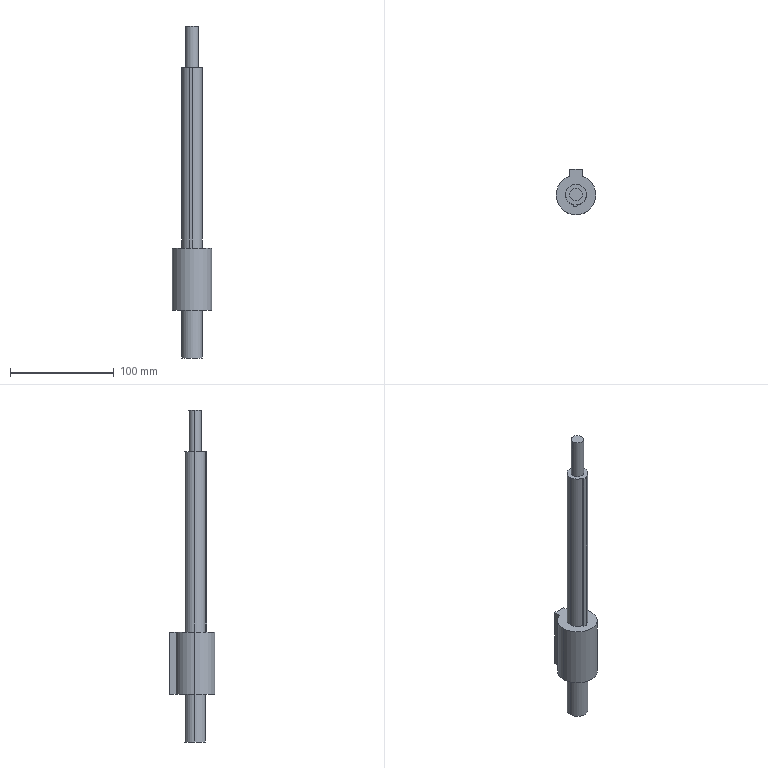Part | STEP file | Camshaft | 1 solid | 21 faces | box 38.228 x 43.828 x 320 mm | volume 147567 mm3 | plane 11 | cylinder 10 | commonest cylinder face diameters 20 x5 38.228 x3 12 x2
STEP:
#1=CARTESIAN_POINT('',(0.,0.,0.));
#2=DIRECTION('',(0.,0.,1.));
#3=DIRECTION('',(1.,0.,0.));
#4=AXIS2_PLACEMENT_3D('',#1,#2,#3);
#5=CARTESIAN_POINT('',(-50.965,1.642,236.173));
#6=VERTEX_POINT('',#5);
#7=CARTESIAN_POINT('',(-62.965,1.642,236.173));
#8=VERTEX_POINT('',#7);
#9=CARTESIAN_POINT('',(-56.965,1.642,236.173));
#10=DIRECTION('',(0.,0.,1.));
#11=DIRECTION('',(1.,0.,0.));
#12=AXIS2_PLACEMENT_3D('',#9,#10,#11);
#13=CIRCLE('',#12,6.);
#14=CARTESIAN_POINT('',(-56.965,1.642,236.173));
#15=DIRECTION('',(0.,0.,-1.));
#16=DIRECTION('',(-1.,0.,0.));
#17=AXIS2_PLACEMENT_3D('',#14,#15,#16);
#18=CYLINDRICAL_SURFACE('',#17,6.);
#19=CARTESIAN_POINT('',(3.142,0.));
#20=DIRECTION('',(-1.,0.));
#21=VECTOR('',#20,1.);
#22=LINE('',#19,#21);
#23=(GEOMETRIC_REPRESENTATION_CONTEXT(2)PARAMETRIC_REPRESENTATION_CONTEXT()REPRESENTATION_CONTEXT('',''));
#24=DEFINITIONAL_REPRESENTATION('',(#22),#23);
#25=PCURVE('',#18,#24);
#26=CARTESIAN_POINT('',(-56.965,1.642,236.173));
#27=DIRECTION('',(0.,0.,1.));
#28=DIRECTION('',(1.,0.,0.));
#29=AXIS2_PLACEMENT_3D('',#26,#27,#28);
#30=PLANE('',#29);
#31=CARTESIAN_POINT('',(0.,0.));
#32=DIRECTION('',(1.,0.));
#33=AXIS2_PLACEMENT_2D('',#31,#32);
#34=CIRCLE('',#33,6.);
#35=(GEOMETRIC_REPRESENTATION_CONTEXT(2)PARAMETRIC_REPRESENTATION_CONTEXT()REPRESENTATION_CONTEXT('',''));
#36=DEFINITIONAL_REPRESENTATION('',(#34),#35);
#37=PCURVE('',#30,#36);
#38=SURFACE_CURVE('',#13,(#25,#37),.PCURVE_S1.);
#39=EDGE_CURVE('',#6,#8,#38,.T.);
#40=ORIENTED_EDGE('',*,*,#39,.F.);
#41=CARTESIAN_POINT('',(-50.965,1.642,196.173));
#42=VERTEX_POINT('',#41);
#43=CARTESIAN_POINT('',(-50.965,1.642,236.173));
#44=DIRECTION('',(0.,0.,-1.));
#45=VECTOR('',#44,1.);
#46=LINE('',#43,#45);
#47=CARTESIAN_POINT('',(3.142,0.));
#48=DIRECTION('',(0.,1.));
#49=VECTOR('',#48,1.);
#50=LINE('',#47,#49);
#51=(GEOMETRIC_REPRESENTATION_CONTEXT(2)PARAMETRIC_REPRESENTATION_CONTEXT()REPRESENTATION_CONTEXT('',''));
#52=DEFINITIONAL_REPRESENTATION('',(#50),#51);
#53=PCURVE('',#18,#52);
#54=CARTESIAN_POINT('',(-56.965,1.642,236.173));
#55=DIRECTION('',(0.,0.,-1.));
#56=DIRECTION('',(-1.,0.,0.));
#57=AXIS2_PLACEMENT_3D('',#54,#55,#56);
#58=CYLINDRICAL_SURFACE('',#57,6.);
#59=CARTESIAN_POINT('',(3.142,0.));
#60=DIRECTION('',(0.,1.));
#61=VECTOR('',#60,1.);
#62=LINE('',#59,#61);
#63=(GEOMETRIC_REPRESENTATION_CONTEXT(2)PARAMETRIC_REPRESENTATION_CONTEXT()REPRESENTATION_CONTEXT('',''));
#64=DEFINITIONAL_REPRESENTATION('',(#62),#63);
#65=PCURVE('',#58,#64);
#66=SURFACE_CURVE('',#46,(#53,#65),.PCURVE_S1.);
#67=EDGE_CURVE('',#6,#42,#66,.T.);
#68=ORIENTED_EDGE('',*,*,#67,.T.);
#69=CARTESIAN_POINT('',(-62.965,1.642,196.173));
#70=VERTEX_POINT('',#69);
#71=CARTESIAN_POINT('',(-56.965,1.642,196.173));
#72=DIRECTION('',(0.,0.,1.));
#73=DIRECTION('',(1.,0.,0.));
#74=AXIS2_PLACEMENT_3D('',#71,#72,#73);
#75=CIRCLE('',#74,6.);
#76=CARTESIAN_POINT('',(3.142,40.));
#77=DIRECTION('',(-1.,0.));
#78=VECTOR('',#77,1.);
#79=LINE('',#76,#78);
#80=(GEOMETRIC_REPRESENTATION_CONTEXT(2)PARAMETRIC_REPRESENTATION_CONTEXT()REPRESENTATION_CONTEXT('',''));
#81=DEFINITIONAL_REPRESENTATION('',(#79),#80);
#82=PCURVE('',#18,#81);
#83=CARTESIAN_POINT('',(-56.965,1.642,196.173));
#84=DIRECTION('',(0.,0.,1.));
#85=DIRECTION('',(1.,0.,0.));
#86=AXIS2_PLACEMENT_3D('',#83,#84,#85);
#87=PLANE('',#86);
#88=CARTESIAN_POINT('',(0.,0.));
#89=DIRECTION('',(1.,0.));
#90=AXIS2_PLACEMENT_2D('',#88,#89);
#91=CIRCLE('',#90,6.);
#92=(GEOMETRIC_REPRESENTATION_CONTEXT(2)PARAMETRIC_REPRESENTATION_CONTEXT()REPRESENTATION_CONTEXT('',''));
#93=DEFINITIONAL_REPRESENTATION('',(#91),#92);
#94=PCURVE('',#87,#93);
#95=SURFACE_CURVE('',#75,(#82,#94),.PCURVE_S1.);
#96=EDGE_CURVE('',#42,#70,#95,.T.);
#97=ORIENTED_EDGE('',*,*,#96,.T.);
#98=CARTESIAN_POINT('',(-62.965,1.642,236.173));
#99=DIRECTION('',(0.,0.,-1.));
#100=VECTOR('',#99,1.);
#101=LINE('',#98,#100);
#102=CARTESIAN_POINT('',(0.,0.));
#103=DIRECTION('',(0.,1.));
#104=VECTOR('',#103,1.);
#105=LINE('',#102,#104);
#106=(GEOMETRIC_REPRESENTATION_CONTEXT(2)PARAMETRIC_REPRESENTATION_CONTEXT()REPRESENTATION_CONTEXT('',''));
#107=DEFINITIONAL_REPRESENTATION('',(#105),#106);
#108=PCURVE('',#18,#107);
#109=CARTESIAN_POINT('',(6.283,0.));
#110=DIRECTION('',(0.,1.));
#111=VECTOR('',#110,1.);
#112=LINE('',#109,#111);
#113=(GEOMETRIC_REPRESENTATION_CONTEXT(2)PARAMETRIC_REPRESENTATION_CONTEXT()REPRESENTATION_CONTEXT('',''));
#114=DEFINITIONAL_REPRESENTATION('',(#112),#113);
#115=PCURVE('',#58,#114);
#116=SURFACE_CURVE('',#101,(#108,#115),.PCURVE_S1.);
#117=EDGE_CURVE('',#8,#70,#116,.T.);
#118=ORIENTED_EDGE('',*,*,#117,.F.);
#119=EDGE_LOOP('',(#40,#68,#97,#118));
#120=FACE_BOUND('',#119,.T.);
#121=ADVANCED_FACE('',(#120),#18,.T.);
#122=CARTESIAN_POINT('',(-46.965,1.642,22.173));
#123=VERTEX_POINT('',#122);
#124=CARTESIAN_POINT('',(-66.965,1.642,22.173));
#125=VERTEX_POINT('',#124);
#126=CARTESIAN_POINT('',(-56.965,1.642,22.173));
#127=DIRECTION('',(0.,0.,1.));
#128=DIRECTION('',(1.,0.,0.));
#129=AXIS2_PLACEMENT_3D('',#126,#127,#128);
#130=CIRCLE('',#129,10.);
#131=CARTESIAN_POINT('',(-56.965,1.642,-83.827));
#132=DIRECTION('',(0.,0.,1.));
#133=DIRECTION('',(1.,0.,0.));
#134=AXIS2_PLACEMENT_3D('',#131,#132,#133);
#135=CYLINDRICAL_SURFACE('',#134,10.);
#136=CARTESIAN_POINT('',(0.,106.));
#137=DIRECTION('',(1.,0.));
#138=VECTOR('',#137,1.);
#139=LINE('',#136,#138);
#140=(GEOMETRIC_REPRESENTATION_CONTEXT(2)PARAMETRIC_REPRESENTATION_CONTEXT()REPRESENTATION_CONTEXT('',''));
#141=DEFINITIONAL_REPRESENTATION('',(#139),#140);
#142=PCURVE('',#135,#141);
#143=CARTESIAN_POINT('',(-56.965,1.642,22.173));
#144=DIRECTION('',(0.,0.,1.));
#145=DIRECTION('',(1.,0.,0.));
#146=AXIS2_PLACEMENT_3D('',#143,#144,#145);
#147=PLANE('',#146);
#148=CARTESIAN_POINT('',(0.,0.));
#149=DIRECTION('',(1.,0.));
#150=AXIS2_PLACEMENT_2D('',#148,#149);
#151=CIRCLE('',#150,10.);
#152=(GEOMETRIC_REPRESENTATION_CONTEXT(2)PARAMETRIC_REPRESENTATION_CONTEXT()REPRESENTATION_CONTEXT('',''));
#153=DEFINITIONAL_REPRESENTATION('',(#151),#152);
#154=PCURVE('',#147,#153);
#155=SURFACE_CURVE('',#130,(#142,#154),.PCURVE_S1.);
#156=EDGE_CURVE('',#123,#125,#155,.T.);
#157=ORIENTED_EDGE('',*,*,#156,.T.);
#158=CARTESIAN_POINT('',(-66.965,1.642,196.173));
#159=VERTEX_POINT('',#158);
#160=CARTESIAN_POINT('',(-66.965,1.642,-83.827));
#161=DIRECTION('',(0.,0.,1.));
#162=VECTOR('',#161,1.);
#163=LINE('',#160,#162);
#164=CARTESIAN_POINT('',(3.142,0.));
#165=DIRECTION('',(0.,1.));
#166=VECTOR('',#165,1.);
#167=LINE('',#164,#166);
#168=(GEOMETRIC_REPRESENTATION_CONTEXT(2)PARAMETRIC_REPRESENTATION_CONTEXT()REPRESENTATION_CONTEXT('',''));
#169=DEFINITIONAL_REPRESENTATION('',(#167),#168);
#170=PCURVE('',#135,#169);
#171=CARTESIAN_POINT('',(-56.965,1.642,-83.827));
#172=DIRECTION('',(0.,0.,1.));
#173=DIRECTION('',(1.,0.,0.));
#174=AXIS2_PLACEMENT_3D('',#171,#172,#173);
#175=CYLINDRICAL_SURFACE('',#174,10.);
#176=CARTESIAN_POINT('',(3.142,0.));
#177=DIRECTION('',(0.,1.));
#178=VECTOR('',#177,1.);
#179=LINE('',#176,#178);
#180=(GEOMETRIC_REPRESENTATION_CONTEXT(2)PARAMETRIC_REPRESENTATION_CONTEXT()REPRESENTATION_CONTEXT('',''));
#181=DEFINITIONAL_REPRESENTATION('',(#179),#180);
#182=PCURVE('',#175,#181);
#183=SURFACE_CURVE('',#163,(#170,#182),.PCURVE_S1.);
#184=EDGE_CURVE('',#125,#159,#183,.T.);
#185=ORIENTED_EDGE('',*,*,#184,.T.);
#186=CARTESIAN_POINT('',(-46.965,1.642,196.173));
#187=VERTEX_POINT('',#186);
#188=CARTESIAN_POINT('',(-56.965,1.642,196.173));
#189=DIRECTION('',(0.,0.,1.));
#190=DIRECTION('',(1.,0.,0.));
#191=AXIS2_PLACEMENT_3D('',#188,#189,#190);
#192=CIRCLE('',#191,10.);
#193=CARTESIAN_POINT('',(0.,280.));
#194=DIRECTION('',(1.,0.));
#195=VECTOR('',#194,1.);
#196=LINE('',#193,#195);
#197=(GEOMETRIC_REPRESENTATION_CONTEXT(2)PARAMETRIC_REPRESENTATION_CONTEXT()REPRESENTATION_CONTEXT('',''));
#198=DEFINITIONAL_REPRESENTATION('',(#196),#197);
#199=PCURVE('',#135,#198);
#200=CARTESIAN_POINT('',(0.,0.));
#201=DIRECTION('',(1.,0.));
#202=AXIS2_PLACEMENT_2D('',#200,#201);
#203=CIRCLE('',#202,10.);
#204=(GEOMETRIC_REPRESENTATION_CONTEXT(2)PARAMETRIC_REPRESENTATION_CONTEXT()REPRESENTATION_CONTEXT('',''));
#205=DEFINITIONAL_REPRESENTATION('',(#203),#204);
#206=PCURVE('',#87,#205);
#207=SURFACE_CURVE('',#192,(#199,#206),.PCURVE_S1.);
#208=EDGE_CURVE('',#187,#159,#207,.T.);
#209=ORIENTED_EDGE('',*,*,#208,.F.);
#210=CARTESIAN_POINT('',(-46.965,1.642,-83.827));
#211=DIRECTION('',(0.,0.,1.));
#212=VECTOR('',#211,1.);
#213=LINE('',#210,#212);
#214=CARTESIAN_POINT('',(0.,0.));
#215=DIRECTION('',(0.,1.));
#216=VECTOR('',#215,1.);
#217=LINE('',#214,#216);
#218=(GEOMETRIC_REPRESENTATION_CONTEXT(2)PARAMETRIC_REPRESENTATION_CONTEXT()REPRESENTATION_CONTEXT('',''));
#219=DEFINITIONAL_REPRESENTATION('',(#217),#218);
#220=PCURVE('',#135,#219);
#221=CARTESIAN_POINT('',(-56.965,1.642,-83.827));
#222=DIRECTION('',(0.,0.,1.));
#223=DIRECTION('',(1.,0.,0.));
#224=AXIS2_PLACEMENT_3D('',#221,#222,#223);
#225=CYLINDRICAL_SURFACE('',#224,10.);
#226=CARTESIAN_POINT('',(6.283,0.));
#227=DIRECTION('',(0.,1.));
#228=VECTOR('',#227,1.);
#229=LINE('',#226,#228);
#230=(GEOMETRIC_REPRESENTATION_CONTEXT(2)PARAMETRIC_REPRESENTATION_CONTEXT()REPRESENTATION_CONTEXT('',''));
#231=DEFINITIONAL_REPRESENTATION('',(#229),#230);
#232=PCURVE('',#225,#231);
#233=SURFACE_CURVE('',#213,(#220,#232),.PCURVE_S1.);
#234=EDGE_CURVE('',#123,#187,#233,.T.);
#235=ORIENTED_EDGE('',*,*,#234,.F.);
#236=EDGE_LOOP('',(#157,#185,#209,#235));
#237=FACE_BOUND('',#236,.T.);
#238=ADVANCED_FACE('',(#237),#135,.T.);
#239=CARTESIAN_POINT('',(-56.27,-8.334,22.173));
#240=VERTEX_POINT('',#239);
#241=CARTESIAN_POINT('',(-56.965,1.642,22.173));
#242=DIRECTION('',(0.,0.,1.));
#243=DIRECTION('',(1.,0.,0.));
#244=AXIS2_PLACEMENT_3D('',#241,#242,#243);
#245=CIRCLE('',#244,10.);
#246=CARTESIAN_POINT('',(0.,106.));
#247=DIRECTION('',(1.,0.));
#248=VECTOR('',#247,1.);
#249=LINE('',#246,#248);
#250=(GEOMETRIC_REPRESENTATION_CONTEXT(2)PARAMETRIC_REPRESENTATION_CONTEXT()REPRESENTATION_CONTEXT('',''));
#251=DEFINITIONAL_REPRESENTATION('',(#249),#250);
#252=PCURVE('',#225,#251);
#253=CARTESIAN_POINT('',(0.,0.));
#254=DIRECTION('',(1.,0.));
#255=AXIS2_PLACEMENT_2D('',#253,#254);
#256=CIRCLE('',#255,10.);
#257=(GEOMETRIC_REPRESENTATION_CONTEXT(2)PARAMETRIC_REPRESENTATION_CONTEXT()REPRESENTATION_CONTEXT('',''));
#258=DEFINITIONAL_REPRESENTATION('',(#256),#257);
#259=PCURVE('',#147,#258);
#260=SURFACE_CURVE('',#245,(#252,#259),.PCURVE_S1.);
#261=EDGE_CURVE('',#240,#123,#260,.T.);
#262=ORIENTED_EDGE('',*,*,#261,.T.);
#263=ORIENTED_EDGE('',*,*,#234,.T.);
#264=CARTESIAN_POINT('',(-56.27,-8.334,196.173));
#265=VERTEX_POINT('',#264);
#266=CARTESIAN_POINT('',(-56.965,1.642,196.173));
#267=DIRECTION('',(0.,0.,1.));
#268=DIRECTION('',(1.,0.,0.));
#269=AXIS2_PLACEMENT_3D('',#266,#267,#268);
#270=CIRCLE('',#269,10.);
#271=CARTESIAN_POINT('',(0.,280.));
#272=DIRECTION('',(1.,0.));
#273=VECTOR('',#272,1.);
#274=LINE('',#271,#273);
#275=(GEOMETRIC_REPRESENTATION_CONTEXT(2)PARAMETRIC_REPRESENTATION_CONTEXT()REPRESENTATION_CONTEXT('',''));
#276=DEFINITIONAL_REPRESENTATION('',(#274),#275);
#277=PCURVE('',#225,#276);
#278=CARTESIAN_POINT('',(0.,0.));
#279=DIRECTION('',(1.,0.));
#280=AXIS2_PLACEMENT_2D('',#278,#279);
#281=CIRCLE('',#280,10.);
#282=(GEOMETRIC_REPRESENTATION_CONTEXT(2)PARAMETRIC_REPRESENTATION_CONTEXT()REPRESENTATION_CONTEXT('',''));
#283=DEFINITIONAL_REPRESENTATION('',(#281),#282);
#284=PCURVE('',#87,#283);
#285=SURFACE_CURVE('',#270,(#277,#284),.PCURVE_S1.);
#286=EDGE_CURVE('',#265,#187,#285,.T.);
#287=ORIENTED_EDGE('',*,*,#286,.F.);
#288=CARTESIAN_POINT('',(-56.27,-8.334,-83.827));
#289=DIRECTION('',(0.,0.,1.));
#290=VECTOR('',#289,1.);
#291=LINE('',#288,#290);
#292=CARTESIAN_POINT('',(4.782,0.));
#293=DIRECTION('',(0.,1.));
#294=VECTOR('',#293,1.);
#295=LINE('',#292,#294);
#296=(GEOMETRIC_REPRESENTATION_CONTEXT(2)PARAMETRIC_REPRESENTATION_CONTEXT()REPRESENTATION_CONTEXT('',''));
#297=DEFINITIONAL_REPRESENTATION('',(#295),#296);
#298=PCURVE('',#225,#297);
#299=CARTESIAN_POINT('',(-56.401,-9.942,9.172));
#300=DIRECTION('',(0.9967,-0.08093,0.));
#301=DIRECTION('',(0.08093,0.9967,0.));
#302=AXIS2_PLACEMENT_3D('',#299,#300,#301);
#303=PLANE('',#302);
#304=CARTESIAN_POINT('',(1.613,-92.999));
#305=DIRECTION('',(0.,1.));
#306=VECTOR('',#305,1.);
#307=LINE('',#304,#306);
#308=(GEOMETRIC_REPRESENTATION_CONTEXT(2)PARAMETRIC_REPRESENTATION_CONTEXT()REPRESENTATION_CONTEXT('',''));
#309=DEFINITIONAL_REPRESENTATION('',(#307),#308);
#310=PCURVE('',#303,#309);
#311=SURFACE_CURVE('',#291,(#298,#310),.PCURVE_S1.);
#312=EDGE_CURVE('',#240,#265,#311,.T.);
#313=ORIENTED_EDGE('',*,*,#312,.F.);
#314=EDGE_LOOP('',(#262,#263,#287,#313));
#315=FACE_BOUND('',#314,.T.);
#316=ADVANCED_FACE('',(#315),#225,.T.);
#317=CARTESIAN_POINT('',(-46.965,1.642,-83.827));
#318=VERTEX_POINT('',#317);
#319=CARTESIAN_POINT('',(-66.965,1.642,-83.827));
#320=VERTEX_POINT('',#319);
#321=CARTESIAN_POINT('',(-56.965,1.642,-83.827));
#322=DIRECTION('',(0.,0.,1.));
#323=DIRECTION('',(1.,0.,0.));
#324=AXIS2_PLACEMENT_3D('',#321,#322,#323);
#325=CIRCLE('',#324,10.);
#326=CARTESIAN_POINT('',(-56.965,1.642,-83.827));
#327=DIRECTION('',(0.,0.,1.));
#328=DIRECTION('',(1.,0.,0.));
#329=AXIS2_PLACEMENT_3D('',#326,#327,#328);
#330=CYLINDRICAL_SURFACE('',#329,10.);
#331=CARTESIAN_POINT('',(0.,0.));
#332=DIRECTION('',(1.,0.));
#333=VECTOR('',#332,1.);
#334=LINE('',#331,#333);
#335=(GEOMETRIC_REPRESENTATION_CONTEXT(2)PARAMETRIC_REPRESENTATION_CONTEXT()REPRESENTATION_CONTEXT('',''));
#336=DEFINITIONAL_REPRESENTATION('',(#334),#335);
#337=PCURVE('',#330,#336);
#338=CARTESIAN_POINT('',(-56.965,1.642,-83.827));
#339=DIRECTION('',(0.,0.,1.));
#340=DIRECTION('',(1.,0.,0.));
#341=AXIS2_PLACEMENT_3D('',#338,#339,#340);
#342=PLANE('',#341);
#343=CARTESIAN_POINT('',(0.,0.));
#344=DIRECTION('',(1.,0.));
#345=AXIS2_PLACEMENT_2D('',#343,#344);
#346=CIRCLE('',#345,10.);
#347=(GEOMETRIC_REPRESENTATION_CONTEXT(2)PARAMETRIC_REPRESENTATION_CONTEXT()REPRESENTATION_CONTEXT('',''));
#348=DEFINITIONAL_REPRESENTATION('',(#346),#347);
#349=PCURVE('',#342,#348);
#350=SURFACE_CURVE('',#325,(#337,#349),.PCURVE_S1.);
#351=EDGE_CURVE('',#318,#320,#350,.T.);
#352=ORIENTED_EDGE('',*,*,#351,.T.);
#353=CARTESIAN_POINT('',(-66.965,1.642,-37.827));
#354=VERTEX_POINT('',#353);
#355=CARTESIAN_POINT('',(-66.965,1.642,-83.827));
#356=DIRECTION('',(0.,0.,1.));
#357=VECTOR('',#356,1.);
#358=LINE('',#355,#357);
#359=CARTESIAN_POINT('',(3.142,0.));
#360=DIRECTION('',(0.,1.));
#361=VECTOR('',#360,1.);
#362=LINE('',#359,#361);
#363=(GEOMETRIC_REPRESENTATION_CONTEXT(2)PARAMETRIC_REPRESENTATION_CONTEXT()REPRESENTATION_CONTEXT('',''));
#364=DEFINITIONAL_REPRESENTATION('',(#362),#363);
#365=PCURVE('',#330,#364);
#366=CARTESIAN_POINT('',(-56.965,1.642,-83.827));
#367=DIRECTION('',(0.,0.,1.));
#368=DIRECTION('',(1.,0.,0.));
#369=AXIS2_PLACEMENT_3D('',#366,#367,#368);
#370=CYLINDRICAL_SURFACE('',#369,10.);
#371=CARTESIAN_POINT('',(3.142,0.));
#372=DIRECTION('',(0.,1.));
#373=VECTOR('',#372,1.);
#374=LINE('',#371,#373);
#375=(GEOMETRIC_REPRESENTATION_CONTEXT(2)PARAMETRIC_REPRESENTATION_CONTEXT()REPRESENTATION_CONTEXT('',''));
#376=DEFINITIONAL_REPRESENTATION('',(#374),#375);
#377=PCURVE('',#370,#376);
#378=SURFACE_CURVE('',#358,(#365,#377),.PCURVE_S1.);
#379=EDGE_CURVE('',#320,#354,#378,.T.);
#380=ORIENTED_EDGE('',*,*,#379,.T.);
#381=CARTESIAN_POINT('',(-46.965,1.642,-37.827));
#382=VERTEX_POINT('',#381);
#383=CARTESIAN_POINT('',(-56.965,1.642,-37.827));
#384=DIRECTION('',(0.,0.,1.));
#385=DIRECTION('',(1.,0.,0.));
#386=AXIS2_PLACEMENT_3D('',#383,#384,#385);
#387=CIRCLE('',#386,10.);
#388=CARTESIAN_POINT('',(0.,46.));
#389=DIRECTION('',(1.,0.));
#390=VECTOR('',#389,1.);
#391=LINE('',#388,#390);
#392=(GEOMETRIC_REPRESENTATION_CONTEXT(2)PARAMETRIC_REPRESENTATION_CONTEXT()REPRESENTATION_CONTEXT('',''));
#393=DEFINITIONAL_REPRESENTATION('',(#391),#392);
#394=PCURVE('',#330,#393);
#395=CARTESIAN_POINT('',(-56.965,1.642,-37.827));
#396=DIRECTION('',(0.,0.,1.));
#397=DIRECTION('',(1.,0.,0.));
#398=AXIS2_PLACEMENT_3D('',#395,#396,#397);
#399=PLANE('',#398);
#400=CARTESIAN_POINT('',(0.,0.));
#401=DIRECTION('',(1.,0.));
#402=AXIS2_PLACEMENT_2D('',#400,#401);
#403=CIRCLE('',#402,10.);
#404=(GEOMETRIC_REPRESENTATION_CONTEXT(2)PARAMETRIC_REPRESENTATION_CONTEXT()REPRESENTATION_CONTEXT('',''));
#405=DEFINITIONAL_REPRESENTATION('',(#403),#404);
#406=PCURVE('',#399,#405);
#407=SURFACE_CURVE('',#387,(#394,#406),.PCURVE_S1.);
#408=EDGE_CURVE('',#382,#354,#407,.T.);
#409=ORIENTED_EDGE('',*,*,#408,.F.);
#410=CARTESIAN_POINT('',(-46.965,1.642,-83.827));
#411=DIRECTION('',(0.,0.,1.));
#412=VECTOR('',#411,1.);
#413=LINE('',#410,#412);
#414=CARTESIAN_POINT('',(0.,0.));
#415=DIRECTION('',(0.,1.));
#416=VECTOR('',#415,1.);
#417=LINE('',#414,#416);
#418=(GEOMETRIC_REPRESENTATION_CONTEXT(2)PARAMETRIC_REPRESENTATION_CONTEXT()REPRESENTATION_CONTEXT('',''));
#419=DEFINITIONAL_REPRESENTATION('',(#417),#418);
#420=PCURVE('',#330,#419);
#421=CARTESIAN_POINT('',(6.283,0.));
#422=DIRECTION('',(0.,1.));
#423=VECTOR('',#422,1.);
#424=LINE('',#421,#423);
#425=(GEOMETRIC_REPRESENTATION_CONTEXT(2)PARAMETRIC_REPRESENTATION_CONTEXT()REPRESENTATION_CONTEXT('',''));
#426=DEFINITIONAL_REPRESENTATION('',(#424),#425);
#427=PCURVE('',#370,#426);
#428=SURFACE_CURVE('',#413,(#420,#427),.PCURVE_S1.);
#429=EDGE_CURVE('',#318,#382,#428,.T.);
#430=ORIENTED_EDGE('',*,*,#429,.F.);
#431=EDGE_LOOP('',(#352,#380,#409,#430));
#432=FACE_BOUND('',#431,.T.);
#433=ADVANCED_FACE('',(#432),#330,.T.);
#434=CARTESIAN_POINT('',(-37.851,1.642,22.173));
#435=VERTEX_POINT('',#434);
#436=CARTESIAN_POINT('',(-50.965,19.79,22.173));
#437=VERTEX_POINT('',#436);
#438=CARTESIAN_POINT('',(-56.965,1.642,22.173));
#439=DIRECTION('',(0.,0.,1.));
#440=DIRECTION('',(1.,0.,0.));
#441=AXIS2_PLACEMENT_3D('',#438,#439,#440);
#442=CIRCLE('',#441,19.114);
#443=CARTESIAN_POINT('',(-56.965,1.642,22.173));
#444=DIRECTION('',(0.,0.,-1.));
#445=DIRECTION('',(-1.,0.,0.));
#446=AXIS2_PLACEMENT_3D('',#443,#444,#445);
#447=CYLINDRICAL_SURFACE('',#446,19.114);
#448=CARTESIAN_POINT('',(3.142,0.));
#449=DIRECTION('',(-1.,0.));
#450=VECTOR('',#449,1.);
#451=LINE('',#448,#450);
#452=(GEOMETRIC_REPRESENTATION_CONTEXT(2)PARAMETRIC_REPRESENTATION_CONTEXT()REPRESENTATION_CONTEXT('',''));
#453=DEFINITIONAL_REPRESENTATION('',(#451),#452);
#454=PCURVE('',#447,#453);
#455=CARTESIAN_POINT('',(0.,0.));
#456=DIRECTION('',(1.,0.));
#457=AXIS2_PLACEMENT_2D('',#455,#456);
#458=CIRCLE('',#457,19.114);
#459=(GEOMETRIC_REPRESENTATION_CONTEXT(2)PARAMETRIC_REPRESENTATION_CONTEXT()REPRESENTATION_CONTEXT('',''));
#460=DEFINITIONAL_REPRESENTATION('',(#458),#459);
#461=PCURVE('',#147,#460);
#462=SURFACE_CURVE('',#442,(#454,#461),.PCURVE_S1.);
#463=EDGE_CURVE('',#435,#437,#462,.T.);
#464=ORIENTED_EDGE('',*,*,#463,.F.);
#465=CARTESIAN_POINT('',(-37.851,1.642,-37.827));
#466=VERTEX_POINT('',#465);
#467=CARTESIAN_POINT('',(-37.851,1.642,22.173));
#468=DIRECTION('',(0.,0.,-1.));
#469=VECTOR('',#468,1.);
#470=LINE('',#467,#469);
#471=CARTESIAN_POINT('',(3.142,0.));
#472=DIRECTION('',(0.,1.));
#473=VECTOR('',#472,1.);
#474=LINE('',#471,#473);
#475=(GEOMETRIC_REPRESENTATION_CONTEXT(2)PARAMETRIC_REPRESENTATION_CONTEXT()REPRESENTATION_CONTEXT('',''));
#476=DEFINITIONAL_REPRESENTATION('',(#474),#475);
#477=PCURVE('',#447,#476);
#478=CARTESIAN_POINT('',(-56.965,1.642,22.173));
#479=DIRECTION('',(0.,0.,-1.));
#480=DIRECTION('',(-1.,0.,0.));
#481=AXIS2_PLACEMENT_3D('',#478,#479,#480);
#482=CYLINDRICAL_SURFACE('',#481,19.114);
#483=CARTESIAN_POINT('',(3.142,0.));
#484=DIRECTION('',(0.,1.));
#485=VECTOR('',#484,1.);
#486=LINE('',#483,#485);
#487=(GEOMETRIC_REPRESENTATION_CONTEXT(2)PARAMETRIC_REPRESENTATION_CONTEXT()REPRESENTATION_CONTEXT('',''));
#488=DEFINITIONAL_REPRESENTATION('',(#486),#487);
#489=PCURVE('',#482,#488);
#490=SURFACE_CURVE('',#470,(#477,#489),.PCURVE_S1.);
#491=EDGE_CURVE('',#435,#466,#490,.T.);
#492=ORIENTED_EDGE('',*,*,#491,.T.);
#493=CARTESIAN_POINT('',(-50.965,19.79,-37.827));
#494=VERTEX_POINT('',#493);
#495=CARTESIAN_POINT('',(-56.965,1.642,-37.827));
#496=DIRECTION('',(0.,0.,1.));
#497=DIRECTION('',(1.,0.,0.));
#498=AXIS2_PLACEMENT_3D('',#495,#496,#497);
#499=CIRCLE('',#498,19.114);
#500=CARTESIAN_POINT('',(3.142,60.));
#501=DIRECTION('',(-1.,0.));
#502=VECTOR('',#501,1.);
#503=LINE('',#500,#502);
#504=(GEOMETRIC_REPRESENTATION_CONTEXT(2)PARAMETRIC_REPRESENTATION_CONTEXT()REPRESENTATION_CONTEXT('',''));
#505=DEFINITIONAL_REPRESENTATION('',(#503),#504);
#506=PCURVE('',#447,#505);
#507=CARTESIAN_POINT('',(0.,0.));
#508=DIRECTION('',(1.,0.));
#509=AXIS2_PLACEMENT_2D('',#507,#508);
#510=CIRCLE('',#509,19.114);
#511=(GEOMETRIC_REPRESENTATION_CONTEXT(2)PARAMETRIC_REPRESENTATION_CONTEXT()REPRESENTATION_CONTEXT('',''));
#512=DEFINITIONAL_REPRESENTATION('',(#510),#511);
#513=PCURVE('',#399,#512);
#514=SURFACE_CURVE('',#499,(#506,#513),.PCURVE_S1.);
#515=EDGE_CURVE('',#466,#494,#514,.T.);
#516=ORIENTED_EDGE('',*,*,#515,.T.);
#517=CARTESIAN_POINT('',(-50.965,19.79,22.173));
#518=DIRECTION('',(0.,0.,-1.));
#519=VECTOR('',#518,1.);
#520=LINE('',#517,#519);
#521=CARTESIAN_POINT('',(1.89,0.));
#522=DIRECTION('',(0.,1.));
#523=VECTOR('',#522,1.);
#524=LINE('',#521,#523);
#525=(GEOMETRIC_REPRESENTATION_CONTEXT(2)PARAMETRIC_REPRESENTATION_CONTEXT()REPRESENTATION_CONTEXT('',''));
#526=DEFINITIONAL_REPRESENTATION('',(#524),#525);
#527=PCURVE('',#447,#526);
#528=CARTESIAN_POINT('',(-50.965,26.356,22.173));
#529=DIRECTION('',(-1.,0.,0.));
#530=DIRECTION('',(0.,0.,1.));
#531=AXIS2_PLACEMENT_3D('',#528,#529,#530);
#532=PLANE('',#531);
#533=CARTESIAN_POINT('',(0.,-6.566));
#534=DIRECTION('',(-1.,0.));
#535=VECTOR('',#534,1.);
#536=LINE('',#533,#535);
#537=(GEOMETRIC_REPRESENTATION_CONTEXT(2)PARAMETRIC_REPRESENTATION_CONTEXT()REPRESENTATION_CONTEXT('',''));
#538=DEFINITIONAL_REPRESENTATION('',(#536),#537);
#539=PCURVE('',#532,#538);
#540=SURFACE_CURVE('',#520,(#527,#539),.PCURVE_S1.);
#541=EDGE_CURVE('',#437,#494,#540,.T.);
#542=ORIENTED_EDGE('',*,*,#541,.F.);
#543=EDGE_LOOP('',(#464,#492,#516,#542));
#544=FACE_BOUND('',#543,.T.);
#545=ADVANCED_FACE('',(#544),#447,.T.);
#546=ORIENTED_EDGE('',*,*,#491,.F.);
#547=CARTESIAN_POINT('',(-76.079,1.642,22.173));
#548=VERTEX_POINT('',#547);
#549=CARTESIAN_POINT('',(-56.965,1.642,22.173));
#550=DIRECTION('',(0.,0.,1.));
#551=DIRECTION('',(1.,0.,0.));
#552=AXIS2_PLACEMENT_3D('',#549,#550,#551);
#553=CIRCLE('',#552,19.114);
#554=CARTESIAN_POINT('',(9.425,0.));
#555=DIRECTION('',(-1.,0.));
#556=VECTOR('',#555,1.);
#557=LINE('',#554,#556);
#558=(GEOMETRIC_REPRESENTATION_CONTEXT(2)PARAMETRIC_REPRESENTATION_CONTEXT()REPRESENTATION_CONTEXT('',''));
#559=DEFINITIONAL_REPRESENTATION('',(#557),#558);
#560=PCURVE('',#482,#559);
#561=CARTESIAN_POINT('',(0.,0.));
#562=DIRECTION('',(1.,0.));
#563=AXIS2_PLACEMENT_2D('',#561,#562);
#564=CIRCLE('',#563,19.114);
#565=(GEOMETRIC_REPRESENTATION_CONTEXT(2)PARAMETRIC_REPRESENTATION_CONTEXT()REPRESENTATION_CONTEXT('',''));
#566=DEFINITIONAL_REPRESENTATION('',(#564),#565);
#567=PCURVE('',#147,#566);
#568=SURFACE_CURVE('',#553,(#560,#567),.PCURVE_S1.);
#569=EDGE_CURVE('',#548,#435,#568,.T.);
#570=ORIENTED_EDGE('',*,*,#569,.F.);
#571=CARTESIAN_POINT('',(-76.079,1.642,-37.827));
#572=VERTEX_POINT('',#571);
#573=CARTESIAN_POINT('',(-76.079,1.642,22.173));
#574=DIRECTION('',(0.,0.,-1.));
#575=VECTOR('',#574,1.);
#576=LINE('',#573,#575);
#577=CARTESIAN_POINT('',(6.283,0.));
#578=DIRECTION('',(0.,1.));
#579=VECTOR('',#578,1.);
#580=LINE('',#577,#579);
#581=(GEOMETRIC_REPRESENTATION_CONTEXT(2)PARAMETRIC_REPRESENTATION_CONTEXT()REPRESENTATION_CONTEXT('',''));
#582=DEFINITIONAL_REPRESENTATION('',(#580),#581);
#583=PCURVE('',#482,#582);
#584=CARTESIAN_POINT('',(-56.965,1.642,22.173));
#585=DIRECTION('',(0.,0.,-1.));
#586=DIRECTION('',(-1.,0.,0.));
#587=AXIS2_PLACEMENT_3D('',#584,#585,#586);
#588=CYLINDRICAL_SURFACE('',#587,19.114);
#589=CARTESIAN_POINT('',(0.,0.));
#590=DIRECTION('',(0.,1.));
#591=VECTOR('',#590,1.);
#592=LINE('',#589,#591);
#593=(GEOMETRIC_REPRESENTATION_CONTEXT(2)PARAMETRIC_REPRESENTATION_CONTEXT()REPRESENTATION_CONTEXT('',''));
#594=DEFINITIONAL_REPRESENTATION('',(#592),#593);
#595=PCURVE('',#588,#594);
#596=SURFACE_CURVE('',#576,(#583,#595),.PCURVE_S1.);
#597=EDGE_CURVE('',#548,#572,#596,.T.);
#598=ORIENTED_EDGE('',*,*,#597,.T.);
#599=CARTESIAN_POINT('',(-56.965,1.642,-37.827));
#600=DIRECTION('',(0.,0.,1.));
#601=DIRECTION('',(1.,0.,0.));
#602=AXIS2_PLACEMENT_3D('',#599,#600,#601);
#603=CIRCLE('',#602,19.114);
#604=CARTESIAN_POINT('',(9.425,60.));
#605=DIRECTION('',(-1.,0.));
#606=VECTOR('',#605,1.);
#607=LINE('',#604,#606);
#608=(GEOMETRIC_REPRESENTATION_CONTEXT(2)PARAMETRIC_REPRESENTATION_CONTEXT()REPRESENTATION_CONTEXT('',''));
#609=DEFINITIONAL_REPRESENTATION('',(#607),#608);
#610=PCURVE('',#482,#609);
#611=CARTESIAN_POINT('',(0.,0.));
#612=DIRECTION('',(1.,0.));
#613=AXIS2_PLACEMENT_2D('',#611,#612);
#614=CIRCLE('',#613,19.114);
#615=(GEOMETRIC_REPRESENTATION_CONTEXT(2)PARAMETRIC_REPRESENTATION_CONTEXT()REPRESENTATION_CONTEXT('',''));
#616=DEFINITIONAL_REPRESENTATION('',(#614),#615);
#617=PCURVE('',#399,#616);
#618=SURFACE_CURVE('',#603,(#610,#617),.PCURVE_S1.);
#619=EDGE_CURVE('',#572,#466,#618,.T.);
#620=ORIENTED_EDGE('',*,*,#619,.T.);
#621=EDGE_LOOP('',(#546,#570,#598,#620));
#622=FACE_BOUND('',#621,.T.);
#623=ADVANCED_FACE('',(#622),#482,.T.);
#624=ORIENTED_EDGE('',*,*,#286,.T.);
#625=ORIENTED_EDGE('',*,*,#208,.T.);
#626=CARTESIAN_POINT('',(-59.26,-8.091,196.173));
#627=VERTEX_POINT('',#626);
#628=CARTESIAN_POINT('',(-56.965,1.642,196.173));
#629=DIRECTION('',(0.,0.,1.));
#630=DIRECTION('',(1.,0.,0.));
#631=AXIS2_PLACEMENT_3D('',#628,#629,#630);
#632=CIRCLE('',#631,10.);
#633=CARTESIAN_POINT('',(0.,0.));
#634=DIRECTION('',(1.,0.));
#635=AXIS2_PLACEMENT_2D('',#633,#634);
#636=CIRCLE('',#635,10.);
#637=(GEOMETRIC_REPRESENTATION_CONTEXT(2)PARAMETRIC_REPRESENTATION_CONTEXT()REPRESENTATION_CONTEXT('',''));
#638=DEFINITIONAL_REPRESENTATION('',(#636),#637);
#639=PCURVE('',#87,#638);
#640=CARTESIAN_POINT('',(0.,280.));
#641=DIRECTION('',(1.,0.));
#642=VECTOR('',#641,1.);
#643=LINE('',#640,#642);
#644=(GEOMETRIC_REPRESENTATION_CONTEXT(2)PARAMETRIC_REPRESENTATION_CONTEXT()REPRESENTATION_CONTEXT('',''));
#645=DEFINITIONAL_REPRESENTATION('',(#643),#644);
#646=PCURVE('',#175,#645);
#647=SURFACE_CURVE('',#632,(#639,#646),.PCURVE_S1.);
#648=EDGE_CURVE('',#159,#627,#647,.T.);
#649=ORIENTED_EDGE('',*,*,#648,.T.);
#650=CARTESIAN_POINT('',(-59.391,-9.699,196.173));
#651=VERTEX_POINT('',#650);
#652=CARTESIAN_POINT('',(-59.391,-9.699,196.173));
#653=DIRECTION('',(-0.08093,-0.9967,0.));
#654=VECTOR('',#653,1.);
#655=LINE('',#652,#654);
#656=CARTESIAN_POINT('',(-2.426,-11.341));
#657=DIRECTION('',(-0.08093,-0.9967));
#658=VECTOR('',#657,1.);
#659=LINE('',#656,#658);
#660=(GEOMETRIC_REPRESENTATION_CONTEXT(2)PARAMETRIC_REPRESENTATION_CONTEXT()REPRESENTATION_CONTEXT('',''));
#661=DEFINITIONAL_REPRESENTATION('',(#659),#660);
#662=PCURVE('',#87,#661);
#663=CARTESIAN_POINT('',(-59.391,-9.699,9.172));
#664=DIRECTION('',(-0.9967,0.08093,0.));
#665=DIRECTION('',(-0.08093,-0.9967,0.));
#666=AXIS2_PLACEMENT_3D('',#663,#664,#665);
#667=PLANE('',#666);
#668=CARTESIAN_POINT('',(0.,187.001));
#669=DIRECTION('',(1.,0.));
#670=VECTOR('',#669,1.);
#671=LINE('',#668,#670);
#672=(GEOMETRIC_REPRESENTATION_CONTEXT(2)PARAMETRIC_REPRESENTATION_CONTEXT()REPRESENTATION_CONTEXT('',''));
#673=DEFINITIONAL_REPRESENTATION('',(#671),#672);
#674=PCURVE('',#667,#673);
#675=SURFACE_CURVE('',#655,(#662,#674),.PCURVE_S1.);
#676=EDGE_CURVE('',#627,#651,#675,.T.);
#677=ORIENTED_EDGE('',*,*,#676,.T.);
#678=CARTESIAN_POINT('',(-56.401,-9.942,196.173));
#679=VERTEX_POINT('',#678);
#680=CARTESIAN_POINT('',(-56.401,-9.942,196.173));
#681=DIRECTION('',(0.9967,-0.08093,0.));
#682=VECTOR('',#681,1.);
#683=LINE('',#680,#682);
#684=CARTESIAN_POINT('',(0.5644,-11.584));
#685=DIRECTION('',(0.9967,-0.08093));
#686=VECTOR('',#685,1.);
#687=LINE('',#684,#686);
#688=(GEOMETRIC_REPRESENTATION_CONTEXT(2)PARAMETRIC_REPRESENTATION_CONTEXT()REPRESENTATION_CONTEXT('',''));
#689=DEFINITIONAL_REPRESENTATION('',(#687),#688);
#690=PCURVE('',#87,#689);
#691=CARTESIAN_POINT('',(-56.401,-9.942,9.172));
#692=DIRECTION('',(-0.08093,-0.9967,0.));
#693=DIRECTION('',(0.9967,-0.08093,0.));
#694=AXIS2_PLACEMENT_3D('',#691,#692,#693);
#695=PLANE('',#694);
#696=CARTESIAN_POINT('',(0.,187.001));
#697=DIRECTION('',(1.,0.));
#698=VECTOR('',#697,1.);
#699=LINE('',#696,#698);
#700=(GEOMETRIC_REPRESENTATION_CONTEXT(2)PARAMETRIC_REPRESENTATION_CONTEXT()REPRESENTATION_CONTEXT('',''));
#701=DEFINITIONAL_REPRESENTATION('',(#699),#700);
#702=PCURVE('',#695,#701);
#703=SURFACE_CURVE('',#683,(#690,#702),.PCURVE_S1.);
#704=EDGE_CURVE('',#651,#679,#703,.T.);
#705=ORIENTED_EDGE('',*,*,#704,.T.);
#706=CARTESIAN_POINT('',(-56.401,-9.942,196.173));
#707=DIRECTION('',(0.08093,0.9967,0.));
#708=VECTOR('',#707,1.);
#709=LINE('',#706,#708);
#710=CARTESIAN_POINT('',(0.5644,-11.584));
#711=DIRECTION('',(0.08093,0.9967));
#712=VECTOR('',#711,1.);
#713=LINE('',#710,#712);
#714=(GEOMETRIC_REPRESENTATION_CONTEXT(2)PARAMETRIC_REPRESENTATION_CONTEXT()REPRESENTATION_CONTEXT('',''));
#715=DEFINITIONAL_REPRESENTATION('',(#713),#714);
#716=PCURVE('',#87,#715);
#717=CARTESIAN_POINT('',(0.,187.001));
#718=DIRECTION('',(1.,0.));
#719=VECTOR('',#718,1.);
#720=LINE('',#717,#719);
#721=(GEOMETRIC_REPRESENTATION_CONTEXT(2)PARAMETRIC_REPRESENTATION_CONTEXT()REPRESENTATION_CONTEXT('',''));
#722=DEFINITIONAL_REPRESENTATION('',(#720),#721);
#723=PCURVE('',#303,#722);
#724=SURFACE_CURVE('',#709,(#716,#723),.PCURVE_S1.);
#725=EDGE_CURVE('',#679,#265,#724,.T.);
#726=ORIENTED_EDGE('',*,*,#725,.T.);
#727=EDGE_LOOP('',(#624,#625,#649,#677,#705,#726));
#728=FACE_BOUND('',#727,.T.);
#729=CARTESIAN_POINT('',(-56.965,1.642,196.173));
#730=DIRECTION('',(0.,0.,1.));
#731=DIRECTION('',(1.,0.,0.));
#732=AXIS2_PLACEMENT_3D('',#729,#730,#731);
#733=CIRCLE('',#732,6.);
#734=CARTESIAN_POINT('',(0.,0.));
#735=DIRECTION('',(1.,0.));
#736=AXIS2_PLACEMENT_2D('',#734,#735);
#737=CIRCLE('',#736,6.);
#738=(GEOMETRIC_REPRESENTATION_CONTEXT(2)PARAMETRIC_REPRESENTATION_CONTEXT()REPRESENTATION_CONTEXT('',''));
#739=DEFINITIONAL_REPRESENTATION('',(#737),#738);
#740=PCURVE('',#87,#739);
#741=CARTESIAN_POINT('',(9.425,40.));
#742=DIRECTION('',(-1.,0.));
#743=VECTOR('',#742,1.);
#744=LINE('',#741,#743);
#745=(GEOMETRIC_REPRESENTATION_CONTEXT(2)PARAMETRIC_REPRESENTATION_CONTEXT()REPRESENTATION_CONTEXT('',''));
#746=DEFINITIONAL_REPRESENTATION('',(#744),#745);
#747=PCURVE('',#58,#746);
#748=SURFACE_CURVE('',#733,(#740,#747),.PCURVE_S1.);
#749=EDGE_CURVE('',#70,#42,#748,.T.);
#750=ORIENTED_EDGE('',*,*,#749,.F.);
#751=ORIENTED_EDGE('',*,*,#96,.F.);
#752=EDGE_LOOP('',(#750,#751));
#753=FACE_BOUND('',#752,.T.);
#754=ADVANCED_FACE('',(#728,#753),#87,.T.);
#755=CARTESIAN_POINT('',(-50.965,26.356,-37.827));
#756=VERTEX_POINT('',#755);
#757=CARTESIAN_POINT('',(-62.965,26.356,-37.827));
#758=VERTEX_POINT('',#757);
#759=CARTESIAN_POINT('',(-62.965,26.356,-37.827));
#760=DIRECTION('',(-1.,0.,0.));
#761=VECTOR('',#760,1.);
#762=LINE('',#759,#761);
#763=CARTESIAN_POINT('',(-62.965,26.356,22.173));
#764=DIRECTION('',(0.,-1.,0.));
#765=DIRECTION('',(0.,0.,-1.));
#766=AXIS2_PLACEMENT_3D('',#763,#764,#765);
#767=PLANE('',#766);
#768=CARTESIAN_POINT('',(60.,0.));
#769=DIRECTION('',(0.,-1.));
#770=VECTOR('',#769,1.);
#771=LINE('',#768,#770);
#772=(GEOMETRIC_REPRESENTATION_CONTEXT(2)PARAMETRIC_REPRESENTATION_CONTEXT()REPRESENTATION_CONTEXT('',''));
#773=DEFINITIONAL_REPRESENTATION('',(#771),#772);
#774=PCURVE('',#767,#773);
#775=CARTESIAN_POINT('',(-6.,24.714));
#776=DIRECTION('',(-1.,0.));
#777=VECTOR('',#776,1.);
#778=LINE('',#775,#777);
#779=(GEOMETRIC_REPRESENTATION_CONTEXT(2)PARAMETRIC_REPRESENTATION_CONTEXT()REPRESENTATION_CONTEXT('',''));
#780=DEFINITIONAL_REPRESENTATION('',(#778),#779);
#781=PCURVE('',#399,#780);
#782=SURFACE_CURVE('',#762,(#774,#781),.PCURVE_S1.);
#783=EDGE_CURVE('',#756,#758,#782,.T.);
#784=ORIENTED_EDGE('',*,*,#783,.T.);
#785=CARTESIAN_POINT('',(-62.965,26.356,22.173));
#786=VERTEX_POINT('',#785);
#787=CARTESIAN_POINT('',(-62.965,26.356,22.173));
#788=DIRECTION('',(0.,0.,-1.));
#789=VECTOR('',#788,1.);
#790=LINE('',#787,#789);
#791=CARTESIAN_POINT('',(0.,0.));
#792=DIRECTION('',(1.,0.));
#793=VECTOR('',#792,1.);
#794=LINE('',#791,#793);
#795=(GEOMETRIC_REPRESENTATION_CONTEXT(2)PARAMETRIC_REPRESENTATION_CONTEXT()REPRESENTATION_CONTEXT('',''));
#796=DEFINITIONAL_REPRESENTATION('',(#794),#795);
#797=PCURVE('',#767,#796);
#798=CARTESIAN_POINT('',(-62.965,19.79,22.173));
#799=DIRECTION('',(1.,0.,0.));
#800=DIRECTION('',(0.,0.,-1.));
#801=AXIS2_PLACEMENT_3D('',#798,#799,#800);
#802=PLANE('',#801);
#803=CARTESIAN_POINT('',(0.,6.566));
#804=DIRECTION('',(1.,0.));
#805=VECTOR('',#804,1.);
#806=LINE('',#803,#805);
#807=(GEOMETRIC_REPRESENTATION_CONTEXT(2)PARAMETRIC_REPRESENTATION_CONTEXT()REPRESENTATION_CONTEXT('',''));
#808=DEFINITIONAL_REPRESENTATION('',(#806),#807);
#809=PCURVE('',#802,#808);
#810=SURFACE_CURVE('',#790,(#797,#809),.PCURVE_S1.);
#811=EDGE_CURVE('',#786,#758,#810,.T.);
#812=ORIENTED_EDGE('',*,*,#811,.F.);
#813=CARTESIAN_POINT('',(-50.965,26.356,22.173));
#814=VERTEX_POINT('',#813);
#815=CARTESIAN_POINT('',(-62.965,26.356,22.173));
#816=DIRECTION('',(-1.,0.,0.));
#817=VECTOR('',#816,1.);
#818=LINE('',#815,#817);
#819=CARTESIAN_POINT('',(0.,0.));
#820=DIRECTION('',(0.,-1.));
#821=VECTOR('',#820,1.);
#822=LINE('',#819,#821);
#823=(GEOMETRIC_REPRESENTATION_CONTEXT(2)PARAMETRIC_REPRESENTATION_CONTEXT()REPRESENTATION_CONTEXT('',''));
#824=DEFINITIONAL_REPRESENTATION('',(#822),#823);
#825=PCURVE('',#767,#824);
#826=CARTESIAN_POINT('',(-6.,24.714));
#827=DIRECTION('',(-1.,0.));
#828=VECTOR('',#827,1.);
#829=LINE('',#826,#828);
#830=(GEOMETRIC_REPRESENTATION_CONTEXT(2)PARAMETRIC_REPRESENTATION_CONTEXT()REPRESENTATION_CONTEXT('',''));
#831=DEFINITIONAL_REPRESENTATION('',(#829),#830);
#832=PCURVE('',#147,#831);
#833=SURFACE_CURVE('',#818,(#825,#832),.PCURVE_S1.);
#834=EDGE_CURVE('',#814,#786,#833,.T.);
#835=ORIENTED_EDGE('',*,*,#834,.F.);
#836=CARTESIAN_POINT('',(-50.965,26.356,22.173));
#837=DIRECTION('',(0.,0.,-1.));
#838=VECTOR('',#837,1.);
#839=LINE('',#836,#838);
#840=CARTESIAN_POINT('',(0.,12.));
#841=DIRECTION('',(1.,0.));
#842=VECTOR('',#841,1.);
#843=LINE('',#840,#842);
#844=(GEOMETRIC_REPRESENTATION_CONTEXT(2)PARAMETRIC_REPRESENTATION_CONTEXT()REPRESENTATION_CONTEXT('',''));
#845=DEFINITIONAL_REPRESENTATION('',(#843),#844);
#846=PCURVE('',#767,#845);
#847=CARTESIAN_POINT('',(0.,0.));
#848=DIRECTION('',(-1.,0.));
#849=VECTOR('',#848,1.);
#850=LINE('',#847,#849);
#851=(GEOMETRIC_REPRESENTATION_CONTEXT(2)PARAMETRIC_REPRESENTATION_CONTEXT()REPRESENTATION_CONTEXT('',''));
#852=DEFINITIONAL_REPRESENTATION('',(#850),#851);
#853=PCURVE('',#532,#852);
#854=SURFACE_CURVE('',#839,(#846,#853),.PCURVE_S1.);
#855=EDGE_CURVE('',#814,#756,#854,.T.);
#856=ORIENTED_EDGE('',*,*,#855,.T.);
#857=EDGE_LOOP('',(#784,#812,#835,#856));
#858=FACE_BOUND('',#857,.T.);
#859=ADVANCED_FACE('',(#858),#767,.F.);
#860=CARTESIAN_POINT('',(-62.965,19.79,-37.827));
#861=VERTEX_POINT('',#860);
#862=CARTESIAN_POINT('',(-62.965,19.79,-37.827));
#863=DIRECTION('',(0.,-1.,0.));
#864=VECTOR('',#863,1.);
#865=LINE('',#862,#864);
#866=CARTESIAN_POINT('',(60.,0.));
#867=DIRECTION('',(0.,-1.));
#868=VECTOR('',#867,1.);
#869=LINE('',#866,#868);
#870=(GEOMETRIC_REPRESENTATION_CONTEXT(2)PARAMETRIC_REPRESENTATION_CONTEXT()REPRESENTATION_CONTEXT('',''));
#871=DEFINITIONAL_REPRESENTATION('',(#869),#870);
#872=PCURVE('',#802,#871);
#873=CARTESIAN_POINT('',(-6.,18.148));
#874=DIRECTION('',(0.,-1.));
#875=VECTOR('',#874,1.);
#876=LINE('',#873,#875);
#877=(GEOMETRIC_REPRESENTATION_CONTEXT(2)PARAMETRIC_REPRESENTATION_CONTEXT()REPRESENTATION_CONTEXT('',''));
#878=DEFINITIONAL_REPRESENTATION('',(#876),#877);
#879=PCURVE('',#399,#878);
#880=SURFACE_CURVE('',#865,(#872,#879),.PCURVE_S1.);
#881=EDGE_CURVE('',#758,#861,#880,.T.);
#882=ORIENTED_EDGE('',*,*,#881,.T.);
#883=CARTESIAN_POINT('',(-62.965,19.79,22.173));
#884=VERTEX_POINT('',#883);
#885=CARTESIAN_POINT('',(-62.965,19.79,22.173));
#886=DIRECTION('',(0.,0.,-1.));
#887=VECTOR('',#886,1.);
#888=LINE('',#885,#887);
#889=CARTESIAN_POINT('',(0.,0.));
#890=DIRECTION('',(1.,0.));
#891=VECTOR('',#890,1.);
#892=LINE('',#889,#891);
#893=(GEOMETRIC_REPRESENTATION_CONTEXT(2)PARAMETRIC_REPRESENTATION_CONTEXT()REPRESENTATION_CONTEXT('',''));
#894=DEFINITIONAL_REPRESENTATION('',(#892),#893);
#895=PCURVE('',#802,#894);
#896=CARTESIAN_POINT('',(1.251,0.));
#897=DIRECTION('',(0.,1.));
#898=VECTOR('',#897,1.);
#899=LINE('',#896,#898);
#900=(GEOMETRIC_REPRESENTATION_CONTEXT(2)PARAMETRIC_REPRESENTATION_CONTEXT()REPRESENTATION_CONTEXT('',''));
#901=DEFINITIONAL_REPRESENTATION('',(#899),#900);
#902=PCURVE('',#588,#901);
#903=SURFACE_CURVE('',#888,(#895,#902),.PCURVE_S1.);
#904=EDGE_CURVE('',#884,#861,#903,.T.);
#905=ORIENTED_EDGE('',*,*,#904,.F.);
#906=CARTESIAN_POINT('',(-62.965,19.79,22.173));
#907=DIRECTION('',(0.,-1.,0.));
#908=VECTOR('',#907,1.);
#909=LINE('',#906,#908);
#910=CARTESIAN_POINT('',(0.,0.));
#911=DIRECTION('',(0.,-1.));
#912=VECTOR('',#911,1.);
#913=LINE('',#910,#912);
#914=(GEOMETRIC_REPRESENTATION_CONTEXT(2)PARAMETRIC_REPRESENTATION_CONTEXT()REPRESENTATION_CONTEXT('',''));
#915=DEFINITIONAL_REPRESENTATION('',(#913),#914);
#916=PCURVE('',#802,#915);
#917=CARTESIAN_POINT('',(-6.,18.148));
#918=DIRECTION('',(0.,-1.));
#919=VECTOR('',#918,1.);
#920=LINE('',#917,#919);
#921=(GEOMETRIC_REPRESENTATION_CONTEXT(2)PARAMETRIC_REPRESENTATION_CONTEXT()REPRESENTATION_CONTEXT('',''));
#922=DEFINITIONAL_REPRESENTATION('',(#920),#921);
#923=PCURVE('',#147,#922);
#924=SURFACE_CURVE('',#909,(#916,#923),.PCURVE_S1.);
#925=EDGE_CURVE('',#786,#884,#924,.T.);
#926=ORIENTED_EDGE('',*,*,#925,.F.);
#927=ORIENTED_EDGE('',*,*,#811,.T.);
#928=EDGE_LOOP('',(#882,#905,#926,#927));
#929=FACE_BOUND('',#928,.T.);
#930=ADVANCED_FACE('',(#929),#802,.F.);
#931=ORIENTED_EDGE('',*,*,#597,.F.);
#932=CARTESIAN_POINT('',(-56.965,1.642,22.173));
#933=DIRECTION('',(0.,0.,1.));
#934=DIRECTION('',(1.,0.,0.));
#935=AXIS2_PLACEMENT_3D('',#932,#933,#934);
#936=CIRCLE('',#935,19.114);
#937=CARTESIAN_POINT('',(3.142,0.));
#938=DIRECTION('',(-1.,0.));
#939=VECTOR('',#938,1.);
#940=LINE('',#937,#939);
#941=(GEOMETRIC_REPRESENTATION_CONTEXT(2)PARAMETRIC_REPRESENTATION_CONTEXT()REPRESENTATION_CONTEXT('',''));
#942=DEFINITIONAL_REPRESENTATION('',(#940),#941);
#943=PCURVE('',#588,#942);
#944=CARTESIAN_POINT('',(0.,0.));
#945=DIRECTION('',(1.,0.));
#946=AXIS2_PLACEMENT_2D('',#944,#945);
#947=CIRCLE('',#946,19.114);
#948=(GEOMETRIC_REPRESENTATION_CONTEXT(2)PARAMETRIC_REPRESENTATION_CONTEXT()REPRESENTATION_CONTEXT('',''));
#949=DEFINITIONAL_REPRESENTATION('',(#947),#948);
#950=PCURVE('',#147,#949);
#951=SURFACE_CURVE('',#936,(#943,#950),.PCURVE_S1.);
#952=EDGE_CURVE('',#884,#548,#951,.T.);
#953=ORIENTED_EDGE('',*,*,#952,.F.);
#954=ORIENTED_EDGE('',*,*,#904,.T.);
#955=CARTESIAN_POINT('',(-56.965,1.642,-37.827));
#956=DIRECTION('',(0.,0.,1.));
#957=DIRECTION('',(1.,0.,0.));
#958=AXIS2_PLACEMENT_3D('',#955,#956,#957);
#959=CIRCLE('',#958,19.114);
#960=CARTESIAN_POINT('',(3.142,60.));
#961=DIRECTION('',(-1.,0.));
#962=VECTOR('',#961,1.);
#963=LINE('',#960,#962);
#964=(GEOMETRIC_REPRESENTATION_CONTEXT(2)PARAMETRIC_REPRESENTATION_CONTEXT()REPRESENTATION_CONTEXT('',''));
#965=DEFINITIONAL_REPRESENTATION('',(#963),#964);
#966=PCURVE('',#588,#965);
#967=CARTESIAN_POINT('',(0.,0.));
#968=DIRECTION('',(1.,0.));
#969=AXIS2_PLACEMENT_2D('',#967,#968);
#970=CIRCLE('',#969,19.114);
#971=(GEOMETRIC_REPRESENTATION_CONTEXT(2)PARAMETRIC_REPRESENTATION_CONTEXT()REPRESENTATION_CONTEXT('',''));
#972=DEFINITIONAL_REPRESENTATION('',(#970),#971);
#973=PCURVE('',#399,#972);
#974=SURFACE_CURVE('',#959,(#966,#973),.PCURVE_S1.);
#975=EDGE_CURVE('',#861,#572,#974,.T.);
#976=ORIENTED_EDGE('',*,*,#975,.T.);
#977=EDGE_LOOP('',(#931,#953,#954,#976));
#978=FACE_BOUND('',#977,.T.);
#979=ADVANCED_FACE('',(#978),#588,.T.);
#980=CARTESIAN_POINT('',(-50.965,26.356,-37.827));
#981=DIRECTION('',(0.,1.,0.));
#982=VECTOR('',#981,1.);
#983=LINE('',#980,#982);
#984=CARTESIAN_POINT('',(-60.,0.));
#985=DIRECTION('',(0.,1.));
#986=VECTOR('',#985,1.);
#987=LINE('',#984,#986);
#988=(GEOMETRIC_REPRESENTATION_CONTEXT(2)PARAMETRIC_REPRESENTATION_CONTEXT()REPRESENTATION_CONTEXT('',''));
#989=DEFINITIONAL_REPRESENTATION('',(#987),#988);
#990=PCURVE('',#532,#989);
#991=CARTESIAN_POINT('',(6.,24.714));
#992=DIRECTION('',(0.,1.));
#993=VECTOR('',#992,1.);
#994=LINE('',#991,#993);
#995=(GEOMETRIC_REPRESENTATION_CONTEXT(2)PARAMETRIC_REPRESENTATION_CONTEXT()REPRESENTATION_CONTEXT('',''));
#996=DEFINITIONAL_REPRESENTATION('',(#994),#995);
#997=PCURVE('',#399,#996);
#998=SURFACE_CURVE('',#983,(#990,#997),.PCURVE_S1.);
#999=EDGE_CURVE('',#494,#756,#998,.T.);
#1000=ORIENTED_EDGE('',*,*,#999,.T.);
#1001=ORIENTED_EDGE('',*,*,#855,.F.);
#1002=CARTESIAN_POINT('',(-50.965,26.356,22.173));
#1003=DIRECTION('',(0.,1.,0.));
#1004=VECTOR('',#1003,1.);
#1005=LINE('',#1002,#1004);
#1006=CARTESIAN_POINT('',(0.,0.));
#1007=DIRECTION('',(0.,1.));
#1008=VECTOR('',#1007,1.);
#1009=LINE('',#1006,#1008);
#1010=(GEOMETRIC_REPRESENTATION_CONTEXT(2)PARAMETRIC_REPRESENTATION_CONTEXT()REPRESENTATION_CONTEXT('',''));
#1011=DEFINITIONAL_REPRESENTATION('',(#1009),#1010);
#1012=PCURVE('',#532,#1011);
#1013=CARTESIAN_POINT('',(6.,24.714));
#1014=DIRECTION('',(0.,1.));
#1015=VECTOR('',#1014,1.);
#1016=LINE('',#1013,#1015);
#1017=(GEOMETRIC_REPRESENTATION_CONTEXT(2)PARAMETRIC_REPRESENTATION_CONTEXT()REPRESENTATION_CONTEXT('',''));
#1018=DEFINITIONAL_REPRESENTATION('',(#1016),#1017);
#1019=PCURVE('',#147,#1018);
#1020=SURFACE_CURVE('',#1005,(#1012,#1019),.PCURVE_S1.);
#1021=EDGE_CURVE('',#437,#814,#1020,.T.);
#1022=ORIENTED_EDGE('',*,*,#1021,.F.);
#1023=ORIENTED_EDGE('',*,*,#541,.T.);
#1024=EDGE_LOOP('',(#1000,#1001,#1022,#1023));
#1025=FACE_BOUND('',#1024,.T.);
#1026=ADVANCED_FACE('',(#1025),#532,.F.);
#1027=CARTESIAN_POINT('',(-56.401,-9.942,22.173));
#1028=VERTEX_POINT('',#1027);
#1029=CARTESIAN_POINT('',(-55.47,1.521,22.173));
#1030=DIRECTION('',(0.08093,0.9967,0.));
#1031=VECTOR('',#1030,1.);
#1032=LINE('',#1029,#1031);
#1033=CARTESIAN_POINT('',(1.495,-0.1214));
#1034=DIRECTION('',(0.08093,0.9967));
#1035=VECTOR('',#1034,1.);
#1036=LINE('',#1033,#1035);
#1037=(GEOMETRIC_REPRESENTATION_CONTEXT(2)PARAMETRIC_REPRESENTATION_CONTEXT()REPRESENTATION_CONTEXT('',''));
#1038=DEFINITIONAL_REPRESENTATION('',(#1036),#1037);
#1039=PCURVE('',#147,#1038);
#1040=CARTESIAN_POINT('',(11.5,13.001));
#1041=DIRECTION('',(1.,0.));
#1042=VECTOR('',#1041,1.);
#1043=LINE('',#1040,#1042);
#1044=(GEOMETRIC_REPRESENTATION_CONTEXT(2)PARAMETRIC_REPRESENTATION_CONTEXT()REPRESENTATION_CONTEXT('',''));
#1045=DEFINITIONAL_REPRESENTATION('',(#1043),#1044);
#1046=PCURVE('',#303,#1045);
#1047=SURFACE_CURVE('',#1032,(#1039,#1046),.PCURVE_S1.);
#1048=EDGE_CURVE('',#1028,#240,#1047,.T.);
#1049=ORIENTED_EDGE('',*,*,#1048,.F.);
#1050=CARTESIAN_POINT('',(-59.391,-9.699,22.173));
#1051=VERTEX_POINT('',#1050);
#1052=CARTESIAN_POINT('',(-57.896,-9.82,22.173));
#1053=DIRECTION('',(0.9967,-0.08093,0.));
#1054=VECTOR('',#1053,1.);
#1055=LINE('',#1052,#1054);
#1056=CARTESIAN_POINT('',(-0.9306,-11.462));
#1057=DIRECTION('',(0.9967,-0.08093));
#1058=VECTOR('',#1057,1.);
#1059=LINE('',#1056,#1058);
#1060=(GEOMETRIC_REPRESENTATION_CONTEXT(2)PARAMETRIC_REPRESENTATION_CONTEXT()REPRESENTATION_CONTEXT('',''));
#1061=DEFINITIONAL_REPRESENTATION('',(#1059),#1060);
#1062=PCURVE('',#147,#1061);
#1063=CARTESIAN_POINT('',(-1.5,13.001));
#1064=DIRECTION('',(1.,0.));
#1065=VECTOR('',#1064,1.);
#1066=LINE('',#1063,#1065);
#1067=(GEOMETRIC_REPRESENTATION_CONTEXT(2)PARAMETRIC_REPRESENTATION_CONTEXT()REPRESENTATION_CONTEXT('',''));
#1068=DEFINITIONAL_REPRESENTATION('',(#1066),#1067);
#1069=PCURVE('',#695,#1068);
#1070=SURFACE_CURVE('',#1055,(#1062,#1069),.PCURVE_S1.);
#1071=EDGE_CURVE('',#1051,#1028,#1070,.T.);
#1072=ORIENTED_EDGE('',*,*,#1071,.F.);
#1073=CARTESIAN_POINT('',(-59.26,-8.091,22.173));
#1074=VERTEX_POINT('',#1073);
#1075=CARTESIAN_POINT('',(-58.46,1.763,22.173));
#1076=DIRECTION('',(-0.08093,-0.9967,0.));
#1077=VECTOR('',#1076,1.);
#1078=LINE('',#1075,#1077);
#1079=CARTESIAN_POINT('',(-1.495,0.1214));
#1080=DIRECTION('',(-0.08093,-0.9967));
#1081=VECTOR('',#1080,1.);
#1082=LINE('',#1079,#1081);
#1083=(GEOMETRIC_REPRESENTATION_CONTEXT(2)PARAMETRIC_REPRESENTATION_CONTEXT()REPRESENTATION_CONTEXT('',''));
#1084=DEFINITIONAL_REPRESENTATION('',(#1082),#1083);
#1085=PCURVE('',#147,#1084);
#1086=CARTESIAN_POINT('',(-11.5,13.001));
#1087=DIRECTION('',(1.,0.));
#1088=VECTOR('',#1087,1.);
#1089=LINE('',#1086,#1088);
#1090=(GEOMETRIC_REPRESENTATION_CONTEXT(2)PARAMETRIC_REPRESENTATION_CONTEXT()REPRESENTATION_CONTEXT('',''));
#1091=DEFINITIONAL_REPRESENTATION('',(#1089),#1090);
#1092=PCURVE('',#667,#1091);
#1093=SURFACE_CURVE('',#1078,(#1085,#1092),.PCURVE_S1.);
#1094=EDGE_CURVE('',#1074,#1051,#1093,.T.);
#1095=ORIENTED_EDGE('',*,*,#1094,.F.);
#1096=CARTESIAN_POINT('',(-56.965,1.642,22.173));
#1097=DIRECTION('',(0.,0.,1.));
#1098=DIRECTION('',(1.,0.,0.));
#1099=AXIS2_PLACEMENT_3D('',#1096,#1097,#1098);
#1100=CIRCLE('',#1099,10.);
#1101=CARTESIAN_POINT('',(0.,0.));
#1102=DIRECTION('',(1.,0.));
#1103=AXIS2_PLACEMENT_2D('',#1101,#1102);
#1104=CIRCLE('',#1103,10.);
#1105=(GEOMETRIC_REPRESENTATION_CONTEXT(2)PARAMETRIC_REPRESENTATION_CONTEXT()REPRESENTATION_CONTEXT('',''));
#1106=DEFINITIONAL_REPRESENTATION('',(#1104),#1105);
#1107=PCURVE('',#147,#1106);
#1108=CARTESIAN_POINT('',(0.,106.));
#1109=DIRECTION('',(1.,0.));
#1110=VECTOR('',#1109,1.);
#1111=LINE('',#1108,#1110);
#1112=(GEOMETRIC_REPRESENTATION_CONTEXT(2)PARAMETRIC_REPRESENTATION_CONTEXT()REPRESENTATION_CONTEXT('',''));
#1113=DEFINITIONAL_REPRESENTATION('',(#1111),#1112);
#1114=PCURVE('',#175,#1113);
#1115=SURFACE_CURVE('',#1100,(#1107,#1114),.PCURVE_S1.);
#1116=EDGE_CURVE('',#125,#1074,#1115,.T.);
#1117=ORIENTED_EDGE('',*,*,#1116,.F.);
#1118=ORIENTED_EDGE('',*,*,#156,.F.);
#1119=ORIENTED_EDGE('',*,*,#261,.F.);
#1120=EDGE_LOOP('',(#1049,#1072,#1095,#1117,#1118,#1119));
#1121=FACE_BOUND('',#1120,.T.);
#1122=ORIENTED_EDGE('',*,*,#834,.T.);
#1123=ORIENTED_EDGE('',*,*,#925,.T.);
#1124=ORIENTED_EDGE('',*,*,#952,.T.);
#1125=ORIENTED_EDGE('',*,*,#569,.T.);
#1126=ORIENTED_EDGE('',*,*,#463,.T.);
#1127=ORIENTED_EDGE('',*,*,#1021,.T.);
#1128=EDGE_LOOP('',(#1122,#1123,#1124,#1125,#1126,#1127));
#1129=FACE_BOUND('',#1128,.T.);
#1130=ADVANCED_FACE('',(#1121,#1129),#147,.T.);
#1131=ORIENTED_EDGE('',*,*,#408,.T.);
#1132=CARTESIAN_POINT('',(-56.965,1.642,-37.827));
#1133=DIRECTION('',(0.,0.,1.));
#1134=DIRECTION('',(1.,0.,0.));
#1135=AXIS2_PLACEMENT_3D('',#1132,#1133,#1134);
#1136=CIRCLE('',#1135,10.);
#1137=CARTESIAN_POINT('',(0.,0.));
#1138=DIRECTION('',(1.,0.));
#1139=AXIS2_PLACEMENT_2D('',#1137,#1138);
#1140=CIRCLE('',#1139,10.);
#1141=(GEOMETRIC_REPRESENTATION_CONTEXT(2)PARAMETRIC_REPRESENTATION_CONTEXT()REPRESENTATION_CONTEXT('',''));
#1142=DEFINITIONAL_REPRESENTATION('',(#1140),#1141);
#1143=PCURVE('',#399,#1142);
#1144=CARTESIAN_POINT('',(0.,46.));
#1145=DIRECTION('',(1.,0.));
#1146=VECTOR('',#1145,1.);
#1147=LINE('',#1144,#1146);
#1148=(GEOMETRIC_REPRESENTATION_CONTEXT(2)PARAMETRIC_REPRESENTATION_CONTEXT()REPRESENTATION_CONTEXT('',''));
#1149=DEFINITIONAL_REPRESENTATION('',(#1147),#1148);
#1150=PCURVE('',#370,#1149);
#1151=SURFACE_CURVE('',#1136,(#1143,#1150),.PCURVE_S1.);
#1152=EDGE_CURVE('',#354,#382,#1151,.T.);
#1153=ORIENTED_EDGE('',*,*,#1152,.T.);
#1154=EDGE_LOOP('',(#1131,#1153));
#1155=FACE_BOUND('',#1154,.T.);
#1156=ORIENTED_EDGE('',*,*,#783,.F.);
#1157=ORIENTED_EDGE('',*,*,#999,.F.);
#1158=ORIENTED_EDGE('',*,*,#515,.F.);
#1159=ORIENTED_EDGE('',*,*,#619,.F.);
#1160=ORIENTED_EDGE('',*,*,#975,.F.);
#1161=ORIENTED_EDGE('',*,*,#881,.F.);
#1162=EDGE_LOOP('',(#1156,#1157,#1158,#1159,#1160,#1161));
#1163=FACE_BOUND('',#1162,.T.);
#1164=ADVANCED_FACE('',(#1155,#1163),#399,.F.);
#1165=ORIENTED_EDGE('',*,*,#351,.F.);
#1166=CARTESIAN_POINT('',(-56.965,1.642,-83.827));
#1167=DIRECTION('',(0.,0.,1.));
#1168=DIRECTION('',(1.,0.,0.));
#1169=AXIS2_PLACEMENT_3D('',#1166,#1167,#1168);
#1170=CIRCLE('',#1169,10.);
#1171=CARTESIAN_POINT('',(0.,0.));
#1172=DIRECTION('',(1.,0.));
#1173=AXIS2_PLACEMENT_2D('',#1171,#1172);
#1174=CIRCLE('',#1173,10.);
#1175=(GEOMETRIC_REPRESENTATION_CONTEXT(2)PARAMETRIC_REPRESENTATION_CONTEXT()REPRESENTATION_CONTEXT('',''));
#1176=DEFINITIONAL_REPRESENTATION('',(#1174),#1175);
#1177=PCURVE('',#342,#1176);
#1178=CARTESIAN_POINT('',(0.,0.));
#1179=DIRECTION('',(1.,0.));
#1180=VECTOR('',#1179,1.);
#1181=LINE('',#1178,#1180);
#1182=(GEOMETRIC_REPRESENTATION_CONTEXT(2)PARAMETRIC_REPRESENTATION_CONTEXT()REPRESENTATION_CONTEXT('',''));
#1183=DEFINITIONAL_REPRESENTATION('',(#1181),#1182);
#1184=PCURVE('',#370,#1183);
#1185=SURFACE_CURVE('',#1170,(#1177,#1184),.PCURVE_S1.);
#1186=EDGE_CURVE('',#320,#318,#1185,.T.);
#1187=ORIENTED_EDGE('',*,*,#1186,.F.);
#1188=EDGE_LOOP('',(#1165,#1187));
#1189=FACE_BOUND('',#1188,.T.);
#1190=ADVANCED_FACE('',(#1189),#342,.F.);
#1191=ORIENTED_EDGE('',*,*,#379,.F.);
#1192=ORIENTED_EDGE('',*,*,#1186,.T.);
#1193=ORIENTED_EDGE('',*,*,#429,.T.);
#1194=ORIENTED_EDGE('',*,*,#1152,.F.);
#1195=EDGE_LOOP('',(#1191,#1192,#1193,#1194));
#1196=FACE_BOUND('',#1195,.T.);
#1197=ADVANCED_FACE('',(#1196),#370,.T.);
#1198=ORIENTED_EDGE('',*,*,#184,.F.);
#1199=ORIENTED_EDGE('',*,*,#1116,.T.);
#1200=CARTESIAN_POINT('',(-59.26,-8.091,-83.827));
#1201=DIRECTION('',(0.,0.,-1.));
#1202=VECTOR('',#1201,1.);
#1203=LINE('',#1200,#1202);
#1204=CARTESIAN_POINT('',(4.481,0.));
#1205=DIRECTION('',(0.,-1.));
#1206=VECTOR('',#1205,1.);
#1207=LINE('',#1204,#1206);
#1208=(GEOMETRIC_REPRESENTATION_CONTEXT(2)PARAMETRIC_REPRESENTATION_CONTEXT()REPRESENTATION_CONTEXT('',''));
#1209=DEFINITIONAL_REPRESENTATION('',(#1207),#1208);
#1210=PCURVE('',#175,#1209);
#1211=CARTESIAN_POINT('',(-1.613,-92.999));
#1212=DIRECTION('',(0.,-1.));
#1213=VECTOR('',#1212,1.);
#1214=LINE('',#1211,#1213);
#1215=(GEOMETRIC_REPRESENTATION_CONTEXT(2)PARAMETRIC_REPRESENTATION_CONTEXT()REPRESENTATION_CONTEXT('',''));
#1216=DEFINITIONAL_REPRESENTATION('',(#1214),#1215);
#1217=PCURVE('',#667,#1216);
#1218=SURFACE_CURVE('',#1203,(#1210,#1217),.PCURVE_S1.);
#1219=EDGE_CURVE('',#627,#1074,#1218,.T.);
#1220=ORIENTED_EDGE('',*,*,#1219,.F.);
#1221=ORIENTED_EDGE('',*,*,#648,.F.);
#1222=EDGE_LOOP('',(#1198,#1199,#1220,#1221));
#1223=FACE_BOUND('',#1222,.T.);
#1224=ADVANCED_FACE('',(#1223),#175,.T.);
#1225=CARTESIAN_POINT('',(-56.401,-9.942,9.172));
#1226=DIRECTION('',(0.,0.,1.));
#1227=VECTOR('',#1226,1.);
#1228=LINE('',#1225,#1227);
#1229=CARTESIAN_POINT('',(0.,0.));
#1230=DIRECTION('',(0.,1.));
#1231=VECTOR('',#1230,1.);
#1232=LINE('',#1229,#1231);
#1233=(GEOMETRIC_REPRESENTATION_CONTEXT(2)PARAMETRIC_REPRESENTATION_CONTEXT()REPRESENTATION_CONTEXT('',''));
#1234=DEFINITIONAL_REPRESENTATION('',(#1232),#1233);
#1235=PCURVE('',#303,#1234);
#1236=CARTESIAN_POINT('',(0.,0.));
#1237=DIRECTION('',(0.,1.));
#1238=VECTOR('',#1237,1.);
#1239=LINE('',#1236,#1238);
#1240=(GEOMETRIC_REPRESENTATION_CONTEXT(2)PARAMETRIC_REPRESENTATION_CONTEXT()REPRESENTATION_CONTEXT('',''));
#1241=DEFINITIONAL_REPRESENTATION('',(#1239),#1240);
#1242=PCURVE('',#695,#1241);
#1243=SURFACE_CURVE('',#1228,(#1235,#1242),.PCURVE_S1.);
#1244=EDGE_CURVE('',#1028,#679,#1243,.T.);
#1245=ORIENTED_EDGE('',*,*,#1244,.F.);
#1246=ORIENTED_EDGE('',*,*,#1048,.T.);
#1247=ORIENTED_EDGE('',*,*,#312,.T.);
#1248=ORIENTED_EDGE('',*,*,#725,.F.);
#1249=EDGE_LOOP('',(#1245,#1246,#1247,#1248));
#1250=FACE_BOUND('',#1249,.T.);
#1251=ADVANCED_FACE('',(#1250),#303,.T.);
#1252=CARTESIAN_POINT('',(-59.391,-9.699,9.172));
#1253=DIRECTION('',(0.,0.,1.));
#1254=VECTOR('',#1253,1.);
#1255=LINE('',#1252,#1254);
#1256=CARTESIAN_POINT('',(-3.,0.));
#1257=DIRECTION('',(0.,1.));
#1258=VECTOR('',#1257,1.);
#1259=LINE('',#1256,#1258);
#1260=(GEOMETRIC_REPRESENTATION_CONTEXT(2)PARAMETRIC_REPRESENTATION_CONTEXT()REPRESENTATION_CONTEXT('',''));
#1261=DEFINITIONAL_REPRESENTATION('',(#1259),#1260);
#1262=PCURVE('',#695,#1261);
#1263=CARTESIAN_POINT('',(0.,0.));
#1264=DIRECTION('',(0.,1.));
#1265=VECTOR('',#1264,1.);
#1266=LINE('',#1263,#1265);
#1267=(GEOMETRIC_REPRESENTATION_CONTEXT(2)PARAMETRIC_REPRESENTATION_CONTEXT()REPRESENTATION_CONTEXT('',''));
#1268=DEFINITIONAL_REPRESENTATION('',(#1266),#1267);
#1269=PCURVE('',#667,#1268);
#1270=SURFACE_CURVE('',#1255,(#1262,#1269),.PCURVE_S1.);
#1271=EDGE_CURVE('',#1051,#651,#1270,.T.);
#1272=ORIENTED_EDGE('',*,*,#1271,.F.);
#1273=ORIENTED_EDGE('',*,*,#1071,.T.);
#1274=ORIENTED_EDGE('',*,*,#1244,.T.);
#1275=ORIENTED_EDGE('',*,*,#704,.F.);
#1276=EDGE_LOOP('',(#1272,#1273,#1274,#1275));
#1277=FACE_BOUND('',#1276,.T.);
#1278=ADVANCED_FACE('',(#1277),#695,.T.);
#1279=ORIENTED_EDGE('',*,*,#1219,.T.);
#1280=ORIENTED_EDGE('',*,*,#1094,.T.);
#1281=ORIENTED_EDGE('',*,*,#1271,.T.);
#1282=ORIENTED_EDGE('',*,*,#676,.F.);
#1283=EDGE_LOOP('',(#1279,#1280,#1281,#1282));
#1284=FACE_BOUND('',#1283,.T.);
#1285=ADVANCED_FACE('',(#1284),#667,.T.);
#1286=ORIENTED_EDGE('',*,*,#67,.F.);
#1287=CARTESIAN_POINT('',(-56.965,1.642,236.173));
#1288=DIRECTION('',(0.,0.,1.));
#1289=DIRECTION('',(1.,0.,0.));
#1290=AXIS2_PLACEMENT_3D('',#1287,#1288,#1289);
#1291=CIRCLE('',#1290,6.);
#1292=CARTESIAN_POINT('',(9.425,0.));
#1293=DIRECTION('',(-1.,0.));
#1294=VECTOR('',#1293,1.);
#1295=LINE('',#1292,#1294);
#1296=(GEOMETRIC_REPRESENTATION_CONTEXT(2)PARAMETRIC_REPRESENTATION_CONTEXT()REPRESENTATION_CONTEXT('',''));
#1297=DEFINITIONAL_REPRESENTATION('',(#1295),#1296);
#1298=PCURVE('',#58,#1297);
#1299=CARTESIAN_POINT('',(0.,0.));
#1300=DIRECTION('',(1.,0.));
#1301=AXIS2_PLACEMENT_2D('',#1299,#1300);
#1302=CIRCLE('',#1301,6.);
#1303=(GEOMETRIC_REPRESENTATION_CONTEXT(2)PARAMETRIC_REPRESENTATION_CONTEXT()REPRESENTATION_CONTEXT('',''));
#1304=DEFINITIONAL_REPRESENTATION('',(#1302),#1303);
#1305=PCURVE('',#30,#1304);
#1306=SURFACE_CURVE('',#1291,(#1298,#1305),.PCURVE_S1.);
#1307=EDGE_CURVE('',#8,#6,#1306,.T.);
#1308=ORIENTED_EDGE('',*,*,#1307,.F.);
#1309=ORIENTED_EDGE('',*,*,#117,.T.);
#1310=ORIENTED_EDGE('',*,*,#749,.T.);
#1311=EDGE_LOOP('',(#1286,#1308,#1309,#1310));
#1312=FACE_BOUND('',#1311,.T.);
#1313=ADVANCED_FACE('',(#1312),#58,.T.);
#1314=ORIENTED_EDGE('',*,*,#1307,.T.);
#1315=ORIENTED_EDGE('',*,*,#39,.T.);
#1316=EDGE_LOOP('',(#1314,#1315));
#1317=FACE_BOUND('',#1316,.T.);
#1318=ADVANCED_FACE('',(#1317),#30,.T.);
#1319=CLOSED_SHELL('',(#121,#238,#316,#433,#545,#623,#754,#859,#930,#979,#1026,#1130,#1164,#1190,#1197,#1224,#1251,#1278,#1285,#1313,#1318));
#1320=MANIFOLD_SOLID_BREP('',#1319);
#1321=(LENGTH_UNIT()NAMED_UNIT(*)SI_UNIT(.MILLI.,.METRE.));
#1322=UNCERTAINTY_MEASURE_WITH_UNIT(LENGTH_MEASURE(0.0000001),#1321,'','');
#1323=(NAMED_UNIT(*)PLANE_ANGLE_UNIT()SI_UNIT($,.RADIAN.));
#1324=(NAMED_UNIT(*)SI_UNIT($,.STERADIAN.)SOLID_ANGLE_UNIT());
#1325=(GEOMETRIC_REPRESENTATION_CONTEXT(3)GLOBAL_UNCERTAINTY_ASSIGNED_CONTEXT((#1322))GLOBAL_UNIT_ASSIGNED_CONTEXT((#1321,#1323,#1324))REPRESENTATION_CONTEXT('',''));
#1326=ADVANCED_BREP_SHAPE_REPRESENTATION('',(#4,#1320),#1325);